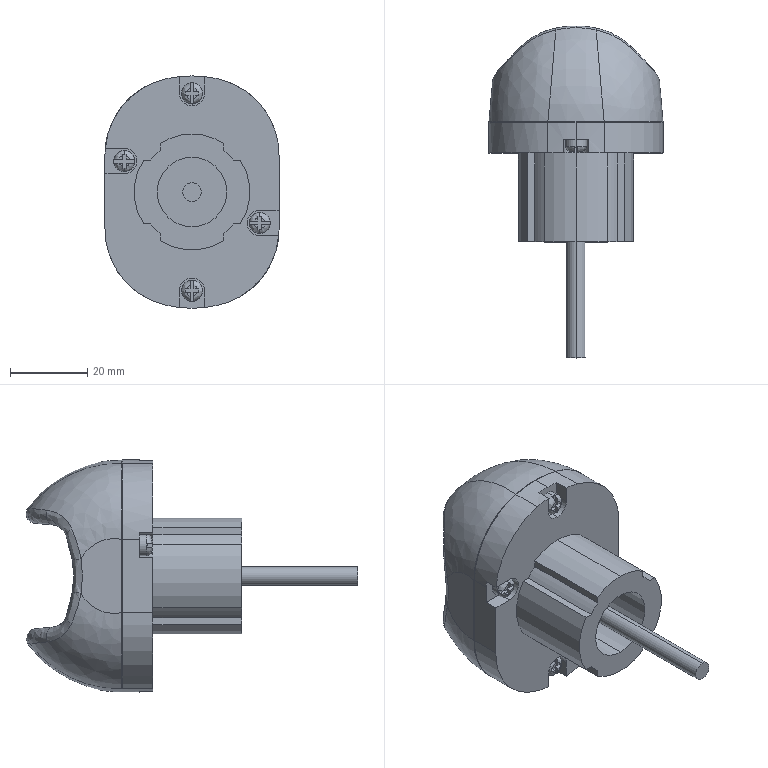Part | SolidWorks | features RefAxis 3, BaseBody 1 | 1 solid | 181 faces | box 45 x 85.792 x 60 mm | volume 63985 mm3 | plane 100 | spline 43 | cylinder 38 | commonest cylinder face diameters 5.5 x8 6.5 x5 30 x5 1 x4 27 x4 59.8 x3